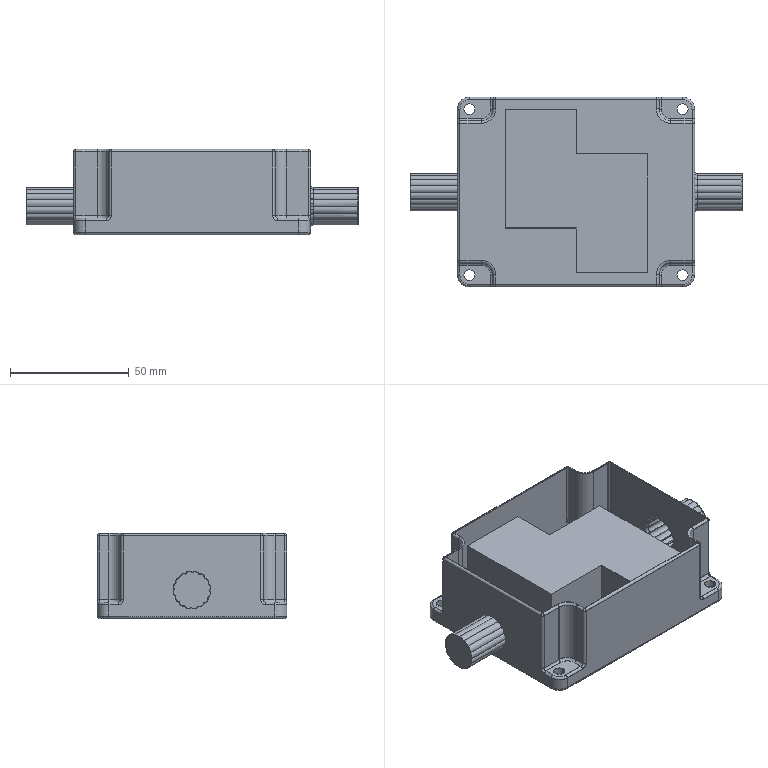Part | SolidWorks | features Boss 2, Cut 2, Extrusion 1, Fillet 1, LPattern 1, Shell 1 | 1 solid | 365 faces | box 140 x 80 x 36 mm | volume 91649 mm3 | cylinder 200 | torus 90 | plane 59 | sphere 16 | commonest cylinder face diameters 3.6 x42 4 x42 2.1 x40 1.7 x32 2.5 x8 4.5 x8